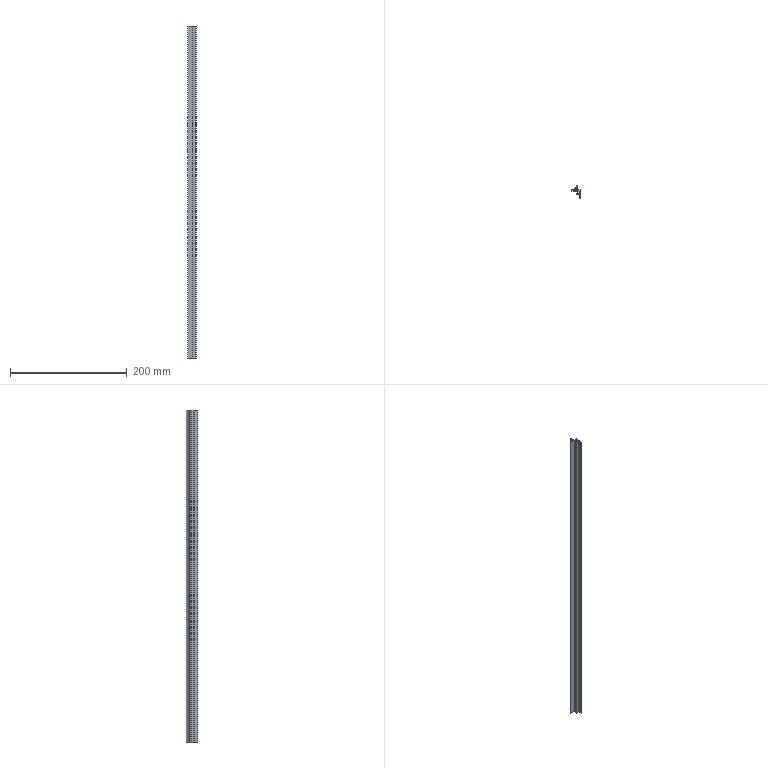Part | SolidWorks | features BaseBody 1, ICE 1, MoveFace 1 | 1 solid | 27 faces | box 14 x 20.3 x 568 mm | volume 28920 mm3 | plane 20 | cylinder 7 | commonest cylinder face diameters 0.387 x2 0.8 x2 0.4 x1 20 x1 22 x1
STEP:
#1=CARTESIAN_POINT('',(-5.304,-0.625,200.));
#2=VERTEX_POINT('',#1);
#3=CARTESIAN_POINT('',(-5.449,-0.8125,200.));
#4=VERTEX_POINT('',#3);
#5=CARTESIAN_POINT('',(-5.255,-0.8125,200.));
#6=DIRECTION('',(0.,0.,1.));
#7=DIRECTION('',(-1.,0.,0.));
#8=AXIS2_PLACEMENT_3D('',#5,#6,#7);
#9=CIRCLE('',#8,0.1937);
#10=EDGE_CURVE('',#2,#4,#9,.T.);
#11=ORIENTED_EDGE('',*,*,#10,.T.);
#12=CARTESIAN_POINT('',(-5.449,-0.8125,-368.));
#13=VERTEX_POINT('',#12);
#14=CARTESIAN_POINT('',(-5.449,-0.8125,230.));
#15=DIRECTION('',(0.,0.,-1.));
#16=VECTOR('',#15,1000.);
#17=LINE('',#14,#16);
#18=EDGE_CURVE('',#4,#13,#17,.T.);
#19=ORIENTED_EDGE('',*,*,#18,.T.);
#20=CARTESIAN_POINT('',(-5.304,-0.625,-368.));
#21=VERTEX_POINT('',#20);
#22=CARTESIAN_POINT('',(-5.255,-0.8125,-368.));
#23=DIRECTION('',(0.,0.,-1.));
#24=DIRECTION('',(1.,0.,0.));
#25=AXIS2_PLACEMENT_3D('',#22,#23,#24);
#26=CIRCLE('',#25,0.1937);
#27=EDGE_CURVE('',#13,#21,#26,.T.);
#28=ORIENTED_EDGE('',*,*,#27,.T.);
#29=CARTESIAN_POINT('',(-5.304,-0.625,230.));
#30=DIRECTION('',(0.,0.,-1.));
#31=VECTOR('',#30,1000.);
#32=LINE('',#29,#31);
#33=EDGE_CURVE('',#2,#21,#32,.T.);
#34=ORIENTED_EDGE('',*,*,#33,.F.);
#35=EDGE_LOOP('',(#11,#19,#28,#34));
#36=FACE_OUTER_BOUND('',#35,.T.);
#37=CARTESIAN_POINT('',(-5.255,-0.8125,230.));
#38=DIRECTION('',(0.,0.,-1.));
#39=DIRECTION('',(-1.,0.,0.));
#40=AXIS2_PLACEMENT_3D('',#37,#38,#39);
#41=CYLINDRICAL_SURFACE('',#40,0.1937);
#42=ADVANCED_FACE('',(#36),#41,.F.);
#43=CARTESIAN_POINT('',(5.,-1.,-368.));
#44=VERTEX_POINT('',#43);
#45=CARTESIAN_POINT('',(5.,-14.3,-368.));
#46=VERTEX_POINT('',#45);
#47=CARTESIAN_POINT('',(5.,29.623,-368.));
#48=DIRECTION('',(0.,-1.,0.));
#49=VECTOR('',#48,1000.);
#50=LINE('',#47,#49);
#51=EDGE_CURVE('',#44,#46,#50,.T.);
#52=ORIENTED_EDGE('',*,*,#51,.F.);
#53=CARTESIAN_POINT('',(5.,-1.,200.));
#54=VERTEX_POINT('',#53);
#55=CARTESIAN_POINT('',(5.,-1.,230.));
#56=DIRECTION('',(0.,0.,-1.));
#57=VECTOR('',#56,1000.);
#58=LINE('',#55,#57);
#59=EDGE_CURVE('',#54,#44,#58,.T.);
#60=ORIENTED_EDGE('',*,*,#59,.F.);
#61=CARTESIAN_POINT('',(5.,-14.3,200.));
#62=VERTEX_POINT('',#61);
#63=CARTESIAN_POINT('',(5.,-14.3,200.));
#64=DIRECTION('',(0.,1.,0.));
#65=VECTOR('',#64,1000.);
#66=LINE('',#63,#65);
#67=EDGE_CURVE('',#62,#54,#66,.T.);
#68=ORIENTED_EDGE('',*,*,#67,.F.);
#69=CARTESIAN_POINT('',(5.,-14.3,230.));
#70=DIRECTION('',(0.,0.,1.));
#71=VECTOR('',#70,1000.);
#72=LINE('',#69,#71);
#73=EDGE_CURVE('',#46,#62,#72,.T.);
#74=ORIENTED_EDGE('',*,*,#73,.F.);
#75=EDGE_LOOP('',(#52,#60,#68,#74));
#76=FACE_OUTER_BOUND('',#75,.T.);
#77=CARTESIAN_POINT('',(5.,-14.3,230.));
#78=DIRECTION('',(-1.,0.,0.));
#79=DIRECTION('',(0.,0.,1.));
#80=AXIS2_PLACEMENT_3D('',#77,#78,#79);
#81=PLANE('',#80);
#82=ADVANCED_FACE('',(#76),#81,.F.);
#83=CARTESIAN_POINT('',(-9.,-2.,-368.));
#84=VERTEX_POINT('',#83);
#85=CARTESIAN_POINT('',(-9.,-2.,200.));
#86=VERTEX_POINT('',#85);
#87=CARTESIAN_POINT('',(-9.,-2.,230.));
#88=DIRECTION('',(0.,0.,1.));
#89=VECTOR('',#88,1000.);
#90=LINE('',#87,#89);
#91=EDGE_CURVE('',#84,#86,#90,.T.);
#92=ORIENTED_EDGE('',*,*,#91,.F.);
#93=CARTESIAN_POINT('',(0.9,-2.,-368.));
#94=VERTEX_POINT('',#93);
#95=CARTESIAN_POINT('',(5.,-2.,-368.));
#96=DIRECTION('',(-1.,0.,0.));
#97=VECTOR('',#96,1000.);
#98=LINE('',#95,#97);
#99=EDGE_CURVE('',#94,#84,#98,.T.);
#100=ORIENTED_EDGE('',*,*,#99,.F.);
#101=CARTESIAN_POINT('',(0.9,-2.,200.));
#102=VERTEX_POINT('',#101);
#103=CARTESIAN_POINT('',(0.9,-2.,230.));
#104=DIRECTION('',(0.,0.,-1.));
#105=VECTOR('',#104,1000.);
#106=LINE('',#103,#105);
#107=EDGE_CURVE('',#102,#94,#106,.T.);
#108=ORIENTED_EDGE('',*,*,#107,.F.);
#109=CARTESIAN_POINT('',(5.,-2.,200.));
#110=DIRECTION('',(1.,0.,0.));
#111=VECTOR('',#110,1000.);
#112=LINE('',#109,#111);
#113=EDGE_CURVE('',#86,#102,#112,.T.);
#114=ORIENTED_EDGE('',*,*,#113,.F.);
#115=EDGE_LOOP('',(#92,#100,#108,#114));
#116=FACE_OUTER_BOUND('',#115,.T.);
#117=CARTESIAN_POINT('',(-9.,-2.,230.));
#118=DIRECTION('',(0.,1.,0.));
#119=DIRECTION('',(0.,0.,1.));
#120=AXIS2_PLACEMENT_3D('',#117,#118,#119);
#121=PLANE('',#120);
#122=ADVANCED_FACE('',(#116),#121,.F.);
#123=CARTESIAN_POINT('',(4.,-6.,200.));
#124=VERTEX_POINT('',#123);
#125=CARTESIAN_POINT('',(4.,-3.,200.));
#126=VERTEX_POINT('',#125);
#127=CARTESIAN_POINT('',(4.,29.623,200.));
#128=DIRECTION('',(0.,1.,0.));
#129=VECTOR('',#128,1000.);
#130=LINE('',#127,#129);
#131=EDGE_CURVE('',#124,#126,#130,.T.);
#132=ORIENTED_EDGE('',*,*,#131,.F.);
#133=CARTESIAN_POINT('',(1.,-6.,200.));
#134=VERTEX_POINT('',#133);
#135=CARTESIAN_POINT('',(5.,-6.,200.));
#136=DIRECTION('',(1.,0.,0.));
#137=VECTOR('',#136,1000.);
#138=LINE('',#135,#137);
#139=EDGE_CURVE('',#134,#124,#138,.T.);
#140=ORIENTED_EDGE('',*,*,#139,.F.);
#141=CARTESIAN_POINT('',(1.,-6.7,200.));
#142=VERTEX_POINT('',#141);
#143=CARTESIAN_POINT('',(1.,-6.,200.));
#144=DIRECTION('',(0.,-1.,0.));
#145=VECTOR('',#144,1000.);
#146=LINE('',#143,#145);
#147=EDGE_CURVE('',#134,#142,#146,.T.);
#148=ORIENTED_EDGE('',*,*,#147,.T.);
#149=CARTESIAN_POINT('',(-1.7,-6.7,200.));
#150=VERTEX_POINT('',#149);
#151=CARTESIAN_POINT('',(5.,-6.7,200.));
#152=DIRECTION('',(1.,0.,0.));
#153=VECTOR('',#152,1000.);
#154=LINE('',#151,#153);
#155=EDGE_CURVE('',#150,#142,#154,.T.);
#156=ORIENTED_EDGE('',*,*,#155,.F.);
#157=CARTESIAN_POINT('',(-1.7,-7.7,200.));
#158=VERTEX_POINT('',#157);
#159=CARTESIAN_POINT('',(-1.7,-6.7,200.));
#160=DIRECTION('',(0.,-1.,0.));
#161=VECTOR('',#160,1000.);
#162=LINE('',#159,#161);
#163=EDGE_CURVE('',#150,#158,#162,.T.);
#164=ORIENTED_EDGE('',*,*,#163,.T.);
#165=CARTESIAN_POINT('',(4.,-7.7,200.));
#166=VERTEX_POINT('',#165);
#167=CARTESIAN_POINT('',(5.,-7.7,200.));
#168=DIRECTION('',(-1.,0.,0.));
#169=VECTOR('',#168,1000.);
#170=LINE('',#167,#169);
#171=EDGE_CURVE('',#166,#158,#170,.T.);
#172=ORIENTED_EDGE('',*,*,#171,.F.);
#173=CARTESIAN_POINT('',(4.,-14.3,200.));
#174=VERTEX_POINT('',#173);
#175=CARTESIAN_POINT('',(4.,29.623,200.));
#176=DIRECTION('',(0.,1.,0.));
#177=VECTOR('',#176,1000.);
#178=LINE('',#175,#177);
#179=EDGE_CURVE('',#174,#166,#178,.T.);
#180=ORIENTED_EDGE('',*,*,#179,.F.);
#181=CARTESIAN_POINT('',(5.,-14.3,200.));
#182=DIRECTION('',(-1.,0.,0.));
#183=VECTOR('',#182,1000.);
#184=LINE('',#181,#183);
#185=EDGE_CURVE('',#62,#174,#184,.T.);
#186=ORIENTED_EDGE('',*,*,#185,.F.);
#187=ORIENTED_EDGE('',*,*,#67,.T.);
#188=CARTESIAN_POINT('',(-5.207,-1.,200.));
#189=VERTEX_POINT('',#188);
#190=CARTESIAN_POINT('',(5.,-1.,200.));
#191=DIRECTION('',(1.,0.,0.));
#192=VECTOR('',#191,1000.);
#193=LINE('',#190,#192);
#194=EDGE_CURVE('',#189,#54,#193,.T.);
#195=ORIENTED_EDGE('',*,*,#194,.F.);
#196=CARTESIAN_POINT('',(-5.255,-0.8125,200.));
#197=DIRECTION('',(0.,0.,1.));
#198=DIRECTION('',(-1.,0.,0.));
#199=AXIS2_PLACEMENT_3D('',#196,#197,#198);
#200=CIRCLE('',#199,0.1937);
#201=EDGE_CURVE('',#4,#189,#200,.T.);
#202=ORIENTED_EDGE('',*,*,#201,.F.);
#203=ORIENTED_EDGE('',*,*,#10,.F.);
#204=CARTESIAN_POINT('',(-1.368,3.063,200.));
#205=VERTEX_POINT('',#204);
#206=CARTESIAN_POINT('',(-10.628,9.,200.));
#207=DIRECTION('',(0.,0.,1.));
#208=DIRECTION('',(-1.,0.,0.));
#209=AXIS2_PLACEMENT_3D('',#206,#207,#208);
#210=CIRCLE('',#209,11.);
#211=EDGE_CURVE('',#2,#205,#210,.T.);
#212=ORIENTED_EDGE('',*,*,#211,.T.);
#213=CARTESIAN_POINT('',(-1.,2.955,200.));
#214=VERTEX_POINT('',#213);
#215=CARTESIAN_POINT('',(-1.2,2.955,200.));
#216=DIRECTION('',(0.,0.,1.));
#217=DIRECTION('',(-1.,0.,0.));
#218=AXIS2_PLACEMENT_3D('',#215,#216,#217);
#219=CIRCLE('',#218,0.2);
#220=EDGE_CURVE('',#214,#205,#219,.T.);
#221=ORIENTED_EDGE('',*,*,#220,.F.);
#222=CARTESIAN_POINT('',(-1.,1.5,200.));
#223=VERTEX_POINT('',#222);
#224=CARTESIAN_POINT('',(-1.,2.955,200.));
#225=DIRECTION('',(0.,1.,0.));
#226=VECTOR('',#225,1000.);
#227=LINE('',#224,#226);
#228=EDGE_CURVE('',#223,#214,#227,.T.);
#229=ORIENTED_EDGE('',*,*,#228,.F.);
#230=CARTESIAN_POINT('',(0.,1.5,200.));
#231=VERTEX_POINT('',#230);
#232=CARTESIAN_POINT('',(-1.,1.5,200.));
#233=DIRECTION('',(-1.,0.,0.));
#234=VECTOR('',#233,1000.);
#235=LINE('',#232,#234);
#236=EDGE_CURVE('',#231,#223,#235,.T.);
#237=ORIENTED_EDGE('',*,*,#236,.F.);
#238=CARTESIAN_POINT('',(0.,6.,200.));
#239=VERTEX_POINT('',#238);
#240=CARTESIAN_POINT('',(0.,1.5,200.));
#241=DIRECTION('',(0.,-1.,0.));
#242=VECTOR('',#241,1000.);
#243=LINE('',#240,#242);
#244=EDGE_CURVE('',#239,#231,#243,.T.);
#245=ORIENTED_EDGE('',*,*,#244,.F.);
#246=CARTESIAN_POINT('',(-0.8,6.,200.));
#247=VERTEX_POINT('',#246);
#248=CARTESIAN_POINT('',(0.,6.,200.));
#249=DIRECTION('',(1.,0.,0.));
#250=VECTOR('',#249,1000.);
#251=LINE('',#248,#250);
#252=EDGE_CURVE('',#247,#239,#251,.T.);
#253=ORIENTED_EDGE('',*,*,#252,.F.);
#254=CARTESIAN_POINT('',(-1.178,5.731,200.));
#255=VERTEX_POINT('',#254);
#256=CARTESIAN_POINT('',(-0.8,5.6,200.));
#257=DIRECTION('',(0.,0.,1.));
#258=DIRECTION('',(-1.,0.,0.));
#259=AXIS2_PLACEMENT_3D('',#256,#257,#258);
#260=CIRCLE('',#259,0.4);
#261=EDGE_CURVE('',#247,#255,#260,.T.);
#262=ORIENTED_EDGE('',*,*,#261,.T.);
#263=CARTESIAN_POINT('',(-8.678,-0.8077,200.));
#264=VERTEX_POINT('',#263);
#265=CARTESIAN_POINT('',(-10.628,9.,200.));
#266=DIRECTION('',(0.,0.,1.));
#267=DIRECTION('',(-1.,0.,0.));
#268=AXIS2_PLACEMENT_3D('',#265,#266,#267);
#269=CIRCLE('',#268,10.);
#270=EDGE_CURVE('',#264,#255,#269,.T.);
#271=ORIENTED_EDGE('',*,*,#270,.F.);
#272=CARTESIAN_POINT('',(-9.,-1.2,200.));
#273=VERTEX_POINT('',#272);
#274=CARTESIAN_POINT('',(-8.6,-1.2,200.));
#275=DIRECTION('',(0.,0.,1.));
#276=DIRECTION('',(-1.,0.,0.));
#277=AXIS2_PLACEMENT_3D('',#274,#275,#276);
#278=CIRCLE('',#277,0.4);
#279=EDGE_CURVE('',#264,#273,#278,.T.);
#280=ORIENTED_EDGE('',*,*,#279,.T.);
#281=CARTESIAN_POINT('',(-9.,8.,200.));
#282=DIRECTION('',(0.,-1.,0.));
#283=VECTOR('',#282,1000.);
#284=LINE('',#281,#283);
#285=EDGE_CURVE('',#273,#86,#284,.T.);
#286=ORIENTED_EDGE('',*,*,#285,.T.);
#287=ORIENTED_EDGE('',*,*,#113,.T.);
#288=CARTESIAN_POINT('',(0.9,-3.,200.));
#289=VERTEX_POINT('',#288);
#290=CARTESIAN_POINT('',(0.9,29.623,200.));
#291=DIRECTION('',(0.,1.,0.));
#292=VECTOR('',#291,1000.);
#293=LINE('',#290,#292);
#294=EDGE_CURVE('',#289,#102,#293,.T.);
#295=ORIENTED_EDGE('',*,*,#294,.F.);
#296=CARTESIAN_POINT('',(5.,-3.,200.));
#297=DIRECTION('',(-1.,0.,0.));
#298=VECTOR('',#297,1000.);
#299=LINE('',#296,#298);
#300=EDGE_CURVE('',#126,#289,#299,.T.);
#301=ORIENTED_EDGE('',*,*,#300,.F.);
#302=EDGE_LOOP('',(#132,#140,#148,#156,#164,#172,#180,#186,#187,#195,#202,#203,#212,#221,#229,#237,#245,#253,#262,#271,#280,#286,#287,#295,#301));
#303=FACE_OUTER_BOUND('',#302,.T.);
#304=CARTESIAN_POINT('',(5.,29.623,200.));
#305=DIRECTION('',(0.,0.,-1.));
#306=DIRECTION('',(-1.,0.,0.));
#307=AXIS2_PLACEMENT_3D('',#304,#305,#306);
#308=PLANE('',#307);
#309=ADVANCED_FACE('',(#303),#308,.F.);
#310=ORIENTED_EDGE('',*,*,#185,.T.);
#311=CARTESIAN_POINT('',(4.,-14.3,-368.));
#312=VERTEX_POINT('',#311);
#313=CARTESIAN_POINT('',(4.,-14.3,230.));
#314=DIRECTION('',(0.,0.,1.));
#315=VECTOR('',#314,1000.);
#316=LINE('',#313,#315);
#317=EDGE_CURVE('',#312,#174,#316,.T.);
#318=ORIENTED_EDGE('',*,*,#317,.F.);
#319=CARTESIAN_POINT('',(5.,-14.3,-368.));
#320=DIRECTION('',(-1.,0.,0.));
#321=VECTOR('',#320,1000.);
#322=LINE('',#319,#321);
#323=EDGE_CURVE('',#46,#312,#322,.T.);
#324=ORIENTED_EDGE('',*,*,#323,.F.);
#325=ORIENTED_EDGE('',*,*,#73,.T.);
#326=EDGE_LOOP('',(#310,#318,#324,#325));
#327=FACE_OUTER_BOUND('',#326,.T.);
#328=CARTESIAN_POINT('',(4.,-14.3,230.));
#329=DIRECTION('',(0.,1.,0.));
#330=DIRECTION('',(0.,0.,1.));
#331=AXIS2_PLACEMENT_3D('',#328,#329,#330);
#332=PLANE('',#331);
#333=ADVANCED_FACE('',(#327),#332,.F.);
#334=ORIENTED_EDGE('',*,*,#51,.T.);
#335=ORIENTED_EDGE('',*,*,#323,.T.);
#336=CARTESIAN_POINT('',(4.,-7.7,-368.));
#337=VERTEX_POINT('',#336);
#338=CARTESIAN_POINT('',(4.,-7.7,-368.));
#339=DIRECTION('',(0.,-1.,0.));
#340=VECTOR('',#339,1000.);
#341=LINE('',#338,#340);
#342=EDGE_CURVE('',#337,#312,#341,.T.);
#343=ORIENTED_EDGE('',*,*,#342,.F.);
#344=CARTESIAN_POINT('',(-1.7,-7.7,-368.));
#345=VERTEX_POINT('',#344);
#346=CARTESIAN_POINT('',(-1.7,-7.7,-368.));
#347=DIRECTION('',(1.,0.,0.));
#348=VECTOR('',#347,1000.);
#349=LINE('',#346,#348);
#350=EDGE_CURVE('',#345,#337,#349,.T.);
#351=ORIENTED_EDGE('',*,*,#350,.F.);
#352=CARTESIAN_POINT('',(-1.7,-6.7,-368.));
#353=VERTEX_POINT('',#352);
#354=CARTESIAN_POINT('',(-1.7,29.623,-368.));
#355=DIRECTION('',(0.,1.,0.));
#356=VECTOR('',#355,1000.);
#357=LINE('',#354,#356);
#358=EDGE_CURVE('',#345,#353,#357,.T.);
#359=ORIENTED_EDGE('',*,*,#358,.T.);
#360=CARTESIAN_POINT('',(1.,-6.7,-368.));
#361=VERTEX_POINT('',#360);
#362=CARTESIAN_POINT('',(1.,-6.7,-368.));
#363=DIRECTION('',(-1.,0.,0.));
#364=VECTOR('',#363,1000.);
#365=LINE('',#362,#364);
#366=EDGE_CURVE('',#361,#353,#365,.T.);
#367=ORIENTED_EDGE('',*,*,#366,.F.);
#368=CARTESIAN_POINT('',(1.,-6.,-368.));
#369=VERTEX_POINT('',#368);
#370=CARTESIAN_POINT('',(1.,29.623,-368.));
#371=DIRECTION('',(0.,1.,0.));
#372=VECTOR('',#371,1000.);
#373=LINE('',#370,#372);
#374=EDGE_CURVE('',#361,#369,#373,.T.);
#375=ORIENTED_EDGE('',*,*,#374,.T.);
#376=CARTESIAN_POINT('',(4.,-6.,-368.));
#377=VERTEX_POINT('',#376);
#378=CARTESIAN_POINT('',(4.,-6.,-368.));
#379=DIRECTION('',(-1.,0.,0.));
#380=VECTOR('',#379,1000.);
#381=LINE('',#378,#380);
#382=EDGE_CURVE('',#377,#369,#381,.T.);
#383=ORIENTED_EDGE('',*,*,#382,.F.);
#384=CARTESIAN_POINT('',(4.,-3.,-368.));
#385=VERTEX_POINT('',#384);
#386=CARTESIAN_POINT('',(4.,-3.,-368.));
#387=DIRECTION('',(0.,-1.,0.));
#388=VECTOR('',#387,1000.);
#389=LINE('',#386,#388);
#390=EDGE_CURVE('',#385,#377,#389,.T.);
#391=ORIENTED_EDGE('',*,*,#390,.F.);
#392=CARTESIAN_POINT('',(0.9,-3.,-368.));
#393=VERTEX_POINT('',#392);
#394=CARTESIAN_POINT('',(0.9,-3.,-368.));
#395=DIRECTION('',(1.,0.,0.));
#396=VECTOR('',#395,1000.);
#397=LINE('',#394,#396);
#398=EDGE_CURVE('',#393,#385,#397,.T.);
#399=ORIENTED_EDGE('',*,*,#398,.F.);
#400=CARTESIAN_POINT('',(0.9,-2.,-368.));
#401=DIRECTION('',(0.,-1.,0.));
#402=VECTOR('',#401,1000.);
#403=LINE('',#400,#402);
#404=EDGE_CURVE('',#94,#393,#403,.T.);
#405=ORIENTED_EDGE('',*,*,#404,.F.);
#406=ORIENTED_EDGE('',*,*,#99,.T.);
#407=CARTESIAN_POINT('',(-9.,-1.2,-368.));
#408=VERTEX_POINT('',#407);
#409=CARTESIAN_POINT('',(-9.,-1.2,-368.));
#410=DIRECTION('',(0.,-1.,0.));
#411=VECTOR('',#410,1000.);
#412=LINE('',#409,#411);
#413=EDGE_CURVE('',#408,#84,#412,.T.);
#414=ORIENTED_EDGE('',*,*,#413,.F.);
#415=CARTESIAN_POINT('',(-8.678,-0.8077,-368.));
#416=VERTEX_POINT('',#415);
#417=CARTESIAN_POINT('',(-8.6,-1.2,-368.));
#418=DIRECTION('',(0.,0.,-1.));
#419=DIRECTION('',(1.,0.,0.));
#420=AXIS2_PLACEMENT_3D('',#417,#418,#419);
#421=CIRCLE('',#420,0.4);
#422=EDGE_CURVE('',#408,#416,#421,.T.);
#423=ORIENTED_EDGE('',*,*,#422,.T.);
#424=CARTESIAN_POINT('',(-1.178,5.731,-368.));
#425=VERTEX_POINT('',#424);
#426=CARTESIAN_POINT('',(-10.628,9.,-368.));
#427=DIRECTION('',(0.,0.,-1.));
#428=DIRECTION('',(1.,0.,0.));
#429=AXIS2_PLACEMENT_3D('',#426,#427,#428);
#430=CIRCLE('',#429,10.);
#431=EDGE_CURVE('',#425,#416,#430,.T.);
#432=ORIENTED_EDGE('',*,*,#431,.F.);
#433=CARTESIAN_POINT('',(-0.8,6.,-368.));
#434=VERTEX_POINT('',#433);
#435=CARTESIAN_POINT('',(-0.8,5.6,-368.));
#436=DIRECTION('',(0.,0.,-1.));
#437=DIRECTION('',(1.,0.,0.));
#438=AXIS2_PLACEMENT_3D('',#435,#436,#437);
#439=CIRCLE('',#438,0.4);
#440=EDGE_CURVE('',#425,#434,#439,.T.);
#441=ORIENTED_EDGE('',*,*,#440,.T.);
#442=CARTESIAN_POINT('',(0.,6.,-368.));
#443=VERTEX_POINT('',#442);
#444=CARTESIAN_POINT('',(0.,6.,-368.));
#445=DIRECTION('',(-1.,0.,0.));
#446=VECTOR('',#445,1000.);
#447=LINE('',#444,#446);
#448=EDGE_CURVE('',#443,#434,#447,.T.);
#449=ORIENTED_EDGE('',*,*,#448,.F.);
#450=CARTESIAN_POINT('',(0.,1.5,-368.));
#451=VERTEX_POINT('',#450);
#452=CARTESIAN_POINT('',(0.,1.5,-368.));
#453=DIRECTION('',(0.,1.,0.));
#454=VECTOR('',#453,1000.);
#455=LINE('',#452,#454);
#456=EDGE_CURVE('',#451,#443,#455,.T.);
#457=ORIENTED_EDGE('',*,*,#456,.F.);
#458=CARTESIAN_POINT('',(-1.,1.5,-368.));
#459=VERTEX_POINT('',#458);
#460=CARTESIAN_POINT('',(-1.,1.5,-368.));
#461=DIRECTION('',(1.,0.,0.));
#462=VECTOR('',#461,1000.);
#463=LINE('',#460,#462);
#464=EDGE_CURVE('',#459,#451,#463,.T.);
#465=ORIENTED_EDGE('',*,*,#464,.F.);
#466=CARTESIAN_POINT('',(-1.,2.955,-368.));
#467=VERTEX_POINT('',#466);
#468=CARTESIAN_POINT('',(-1.,2.955,-368.));
#469=DIRECTION('',(0.,-1.,0.));
#470=VECTOR('',#469,1000.);
#471=LINE('',#468,#470);
#472=EDGE_CURVE('',#467,#459,#471,.T.);
#473=ORIENTED_EDGE('',*,*,#472,.F.);
#474=CARTESIAN_POINT('',(-1.368,3.063,-368.));
#475=VERTEX_POINT('',#474);
#476=CARTESIAN_POINT('',(-1.2,2.955,-368.));
#477=DIRECTION('',(0.,0.,-1.));
#478=DIRECTION('',(1.,0.,0.));
#479=AXIS2_PLACEMENT_3D('',#476,#477,#478);
#480=CIRCLE('',#479,0.2);
#481=EDGE_CURVE('',#475,#467,#480,.T.);
#482=ORIENTED_EDGE('',*,*,#481,.F.);
#483=CARTESIAN_POINT('',(-10.628,9.,-368.));
#484=DIRECTION('',(0.,0.,-1.));
#485=DIRECTION('',(1.,0.,0.));
#486=AXIS2_PLACEMENT_3D('',#483,#484,#485);
#487=CIRCLE('',#486,11.);
#488=EDGE_CURVE('',#475,#21,#487,.T.);
#489=ORIENTED_EDGE('',*,*,#488,.T.);
#490=ORIENTED_EDGE('',*,*,#27,.F.);
#491=CARTESIAN_POINT('',(-5.207,-1.,-368.));
#492=VERTEX_POINT('',#491);
#493=CARTESIAN_POINT('',(-5.255,-0.8125,-368.));
#494=DIRECTION('',(0.,0.,-1.));
#495=DIRECTION('',(1.,0.,0.));
#496=AXIS2_PLACEMENT_3D('',#493,#494,#495);
#497=CIRCLE('',#496,0.1937);
#498=EDGE_CURVE('',#492,#13,#497,.T.);
#499=ORIENTED_EDGE('',*,*,#498,.F.);
#500=CARTESIAN_POINT('',(5.,-1.,-368.));
#501=DIRECTION('',(-1.,0.,0.));
#502=VECTOR('',#501,1000.);
#503=LINE('',#500,#502);
#504=EDGE_CURVE('',#44,#492,#503,.T.);
#505=ORIENTED_EDGE('',*,*,#504,.F.);
#506=EDGE_LOOP('',(#334,#335,#343,#351,#359,#367,#375,#383,#391,#399,#405,#406,#414,#423,#432,#441,#449,#457,#465,#473,#482,#489,#490,#499,#505));
#507=FACE_OUTER_BOUND('',#506,.T.);
#508=CARTESIAN_POINT('',(5.,29.623,-368.));
#509=DIRECTION('',(0.,0.,1.));
#510=DIRECTION('',(1.,0.,0.));
#511=AXIS2_PLACEMENT_3D('',#508,#509,#510);
#512=PLANE('',#511);
#513=ADVANCED_FACE('',(#507),#512,.F.);
#514=ORIENTED_EDGE('',*,*,#59,.T.);
#515=ORIENTED_EDGE('',*,*,#504,.T.);
#516=CARTESIAN_POINT('',(-5.207,-1.,230.));
#517=DIRECTION('',(0.,0.,-1.));
#518=VECTOR('',#517,1000.);
#519=LINE('',#516,#518);
#520=EDGE_CURVE('',#189,#492,#519,.T.);
#521=ORIENTED_EDGE('',*,*,#520,.F.);
#522=ORIENTED_EDGE('',*,*,#194,.T.);
#523=EDGE_LOOP('',(#514,#515,#521,#522));
#524=FACE_OUTER_BOUND('',#523,.T.);
#525=CARTESIAN_POINT('',(5.,-1.,230.));
#526=DIRECTION('',(0.,-1.,0.));
#527=DIRECTION('',(0.,0.,-1.));
#528=AXIS2_PLACEMENT_3D('',#525,#526,#527);
#529=PLANE('',#528);
#530=ADVANCED_FACE('',(#524),#529,.F.);
#531=CARTESIAN_POINT('',(-9.,-1.2,230.));
#532=DIRECTION('',(0.,0.,1.));
#533=VECTOR('',#532,1000.);
#534=LINE('',#531,#533);
#535=EDGE_CURVE('',#408,#273,#534,.T.);
#536=ORIENTED_EDGE('',*,*,#535,.F.);
#537=ORIENTED_EDGE('',*,*,#413,.T.);
#538=ORIENTED_EDGE('',*,*,#91,.T.);
#539=ORIENTED_EDGE('',*,*,#285,.F.);
#540=EDGE_LOOP('',(#536,#537,#538,#539));
#541=FACE_OUTER_BOUND('',#540,.T.);
#542=CARTESIAN_POINT('',(-9.,-1.2,230.));
#543=DIRECTION('',(1.,0.,0.));
#544=DIRECTION('',(0.,0.,-1.));
#545=AXIS2_PLACEMENT_3D('',#542,#543,#544);
#546=PLANE('',#545);
#547=ADVANCED_FACE('',(#541),#546,.F.);
#548=ORIENTED_EDGE('',*,*,#294,.T.);
#549=ORIENTED_EDGE('',*,*,#107,.T.);
#550=ORIENTED_EDGE('',*,*,#404,.T.);
#551=CARTESIAN_POINT('',(0.9,-3.,230.));
#552=DIRECTION('',(0.,0.,-1.));
#553=VECTOR('',#552,1000.);
#554=LINE('',#551,#553);
#555=EDGE_CURVE('',#289,#393,#554,.T.);
#556=ORIENTED_EDGE('',*,*,#555,.F.);
#557=EDGE_LOOP('',(#548,#549,#550,#556));
#558=FACE_OUTER_BOUND('',#557,.T.);
#559=CARTESIAN_POINT('',(0.9,-2.,230.));
#560=DIRECTION('',(1.,0.,0.));
#561=DIRECTION('',(0.,0.,-1.));
#562=AXIS2_PLACEMENT_3D('',#559,#560,#561);
#563=PLANE('',#562);
#564=ADVANCED_FACE('',(#558),#563,.F.);
#565=ORIENTED_EDGE('',*,*,#300,.T.);
#566=ORIENTED_EDGE('',*,*,#555,.T.);
#567=ORIENTED_EDGE('',*,*,#398,.T.);
#568=CARTESIAN_POINT('',(4.,-3.,230.));
#569=DIRECTION('',(0.,0.,-1.));
#570=VECTOR('',#569,1000.);
#571=LINE('',#568,#570);
#572=EDGE_CURVE('',#126,#385,#571,.T.);
#573=ORIENTED_EDGE('',*,*,#572,.F.);
#574=EDGE_LOOP('',(#565,#566,#567,#573));
#575=FACE_OUTER_BOUND('',#574,.T.);
#576=CARTESIAN_POINT('',(0.9,-3.,230.));
#577=DIRECTION('',(0.,1.,0.));
#578=DIRECTION('',(0.,0.,1.));
#579=AXIS2_PLACEMENT_3D('',#576,#577,#578);
#580=PLANE('',#579);
#581=ADVANCED_FACE('',(#575),#580,.F.);
#582=ORIENTED_EDGE('',*,*,#131,.T.);
#583=ORIENTED_EDGE('',*,*,#572,.T.);
#584=ORIENTED_EDGE('',*,*,#390,.T.);
#585=CARTESIAN_POINT('',(4.,-6.,230.));
#586=DIRECTION('',(0.,0.,-1.));
#587=VECTOR('',#586,1000.);
#588=LINE('',#585,#587);
#589=EDGE_CURVE('',#124,#377,#588,.T.);
#590=ORIENTED_EDGE('',*,*,#589,.F.);
#591=EDGE_LOOP('',(#582,#583,#584,#590));
#592=FACE_OUTER_BOUND('',#591,.T.);
#593=CARTESIAN_POINT('',(4.,-3.,230.));
#594=DIRECTION('',(1.,0.,0.));
#595=DIRECTION('',(0.,0.,-1.));
#596=AXIS2_PLACEMENT_3D('',#593,#594,#595);
#597=PLANE('',#596);
#598=ADVANCED_FACE('',(#592),#597,.F.);
#599=ORIENTED_EDGE('',*,*,#139,.T.);
#600=ORIENTED_EDGE('',*,*,#589,.T.);
#601=ORIENTED_EDGE('',*,*,#382,.T.);
#602=CARTESIAN_POINT('',(1.,-6.,230.));
#603=DIRECTION('',(0.,0.,-1.));
#604=VECTOR('',#603,1000.);
#605=LINE('',#602,#604);
#606=EDGE_CURVE('',#134,#369,#605,.T.);
#607=ORIENTED_EDGE('',*,*,#606,.F.);
#608=EDGE_LOOP('',(#599,#600,#601,#607));
#609=FACE_OUTER_BOUND('',#608,.T.);
#610=CARTESIAN_POINT('',(4.,-6.,230.));
#611=DIRECTION('',(0.,-1.,0.));
#612=DIRECTION('',(0.,0.,-1.));
#613=AXIS2_PLACEMENT_3D('',#610,#611,#612);
#614=PLANE('',#613);
#615=ADVANCED_FACE('',(#609),#614,.F.);
#616=ORIENTED_EDGE('',*,*,#155,.T.);
#617=CARTESIAN_POINT('',(1.,-6.7,230.));
#618=DIRECTION('',(0.,0.,1.));
#619=VECTOR('',#618,1000.);
#620=LINE('',#617,#619);
#621=EDGE_CURVE('',#361,#142,#620,.T.);
#622=ORIENTED_EDGE('',*,*,#621,.F.);
#623=ORIENTED_EDGE('',*,*,#366,.T.);
#624=CARTESIAN_POINT('',(-1.7,-6.7,230.));
#625=DIRECTION('',(0.,0.,-1.));
#626=VECTOR('',#625,1000.);
#627=LINE('',#624,#626);
#628=EDGE_CURVE('',#150,#353,#627,.T.);
#629=ORIENTED_EDGE('',*,*,#628,.F.);
#630=EDGE_LOOP('',(#616,#622,#623,#629));
#631=FACE_OUTER_BOUND('',#630,.T.);
#632=CARTESIAN_POINT('',(1.,-6.7,230.));
#633=DIRECTION('',(0.,-1.,0.));
#634=DIRECTION('',(0.,0.,-1.));
#635=AXIS2_PLACEMENT_3D('',#632,#633,#634);
#636=PLANE('',#635);
#637=ADVANCED_FACE('',(#631),#636,.F.);
#638=ORIENTED_EDGE('',*,*,#171,.T.);
#639=CARTESIAN_POINT('',(-1.7,-7.7,230.));
#640=DIRECTION('',(0.,0.,1.));
#641=VECTOR('',#640,1000.);
#642=LINE('',#639,#641);
#643=EDGE_CURVE('',#345,#158,#642,.T.);
#644=ORIENTED_EDGE('',*,*,#643,.F.);
#645=ORIENTED_EDGE('',*,*,#350,.T.);
#646=CARTESIAN_POINT('',(4.,-7.7,230.));
#647=DIRECTION('',(0.,0.,-1.));
#648=VECTOR('',#647,1000.);
#649=LINE('',#646,#648);
#650=EDGE_CURVE('',#166,#337,#649,.T.);
#651=ORIENTED_EDGE('',*,*,#650,.F.);
#652=EDGE_LOOP('',(#638,#644,#645,#651));
#653=FACE_OUTER_BOUND('',#652,.T.);
#654=CARTESIAN_POINT('',(-1.7,-7.7,230.));
#655=DIRECTION('',(0.,1.,0.));
#656=DIRECTION('',(0.,0.,1.));
#657=AXIS2_PLACEMENT_3D('',#654,#655,#656);
#658=PLANE('',#657);
#659=ADVANCED_FACE('',(#653),#658,.F.);
#660=ORIENTED_EDGE('',*,*,#179,.T.);
#661=ORIENTED_EDGE('',*,*,#650,.T.);
#662=ORIENTED_EDGE('',*,*,#342,.T.);
#663=ORIENTED_EDGE('',*,*,#317,.T.);
#664=EDGE_LOOP('',(#660,#661,#662,#663));
#665=FACE_OUTER_BOUND('',#664,.T.);
#666=CARTESIAN_POINT('',(4.,-7.7,230.));
#667=DIRECTION('',(1.,0.,0.));
#668=DIRECTION('',(0.,0.,-1.));
#669=AXIS2_PLACEMENT_3D('',#666,#667,#668);
#670=PLANE('',#669);
#671=ADVANCED_FACE('',(#665),#670,.F.);
#672=ORIENTED_EDGE('',*,*,#18,.F.);
#673=ORIENTED_EDGE('',*,*,#201,.T.);
#674=ORIENTED_EDGE('',*,*,#520,.T.);
#675=ORIENTED_EDGE('',*,*,#498,.T.);
#676=EDGE_LOOP('',(#672,#673,#674,#675));
#677=FACE_OUTER_BOUND('',#676,.T.);
#678=CARTESIAN_POINT('',(-5.255,-0.8125,230.));
#679=DIRECTION('',(0.,0.,-1.));
#680=DIRECTION('',(-1.,0.,0.));
#681=AXIS2_PLACEMENT_3D('',#678,#679,#680);
#682=CYLINDRICAL_SURFACE('',#681,0.1937);
#683=ADVANCED_FACE('',(#677),#682,.F.);
#684=CARTESIAN_POINT('',(-1.,2.955,230.));
#685=DIRECTION('',(0.,0.,1.));
#686=VECTOR('',#685,1000.);
#687=LINE('',#684,#686);
#688=EDGE_CURVE('',#467,#214,#687,.T.);
#689=ORIENTED_EDGE('',*,*,#688,.F.);
#690=ORIENTED_EDGE('',*,*,#472,.T.);
#691=CARTESIAN_POINT('',(-1.,1.5,230.));
#692=DIRECTION('',(0.,0.,-1.));
#693=VECTOR('',#692,1000.);
#694=LINE('',#691,#693);
#695=EDGE_CURVE('',#223,#459,#694,.T.);
#696=ORIENTED_EDGE('',*,*,#695,.F.);
#697=ORIENTED_EDGE('',*,*,#228,.T.);
#698=EDGE_LOOP('',(#689,#690,#696,#697));
#699=FACE_OUTER_BOUND('',#698,.T.);
#700=CARTESIAN_POINT('',(-1.,2.955,230.));
#701=DIRECTION('',(1.,0.,0.));
#702=DIRECTION('',(0.,0.,-1.));
#703=AXIS2_PLACEMENT_3D('',#700,#701,#702);
#704=PLANE('',#703);
#705=ADVANCED_FACE('',(#699),#704,.F.);
#706=ORIENTED_EDGE('',*,*,#488,.F.);
#707=CARTESIAN_POINT('',(-1.368,3.063,230.));
#708=DIRECTION('',(0.,0.,1.));
#709=VECTOR('',#708,1000.);
#710=LINE('',#707,#709);
#711=EDGE_CURVE('',#475,#205,#710,.T.);
#712=ORIENTED_EDGE('',*,*,#711,.T.);
#713=ORIENTED_EDGE('',*,*,#211,.F.);
#714=ORIENTED_EDGE('',*,*,#33,.T.);
#715=EDGE_LOOP('',(#706,#712,#713,#714));
#716=FACE_OUTER_BOUND('',#715,.T.);
#717=CARTESIAN_POINT('',(-10.628,9.,230.));
#718=DIRECTION('',(0.,0.,-1.));
#719=DIRECTION('',(-1.,0.,0.));
#720=AXIS2_PLACEMENT_3D('',#717,#718,#719);
#721=CYLINDRICAL_SURFACE('',#720,11.);
#722=ADVANCED_FACE('',(#716),#721,.T.);
#723=CARTESIAN_POINT('',(-1.178,5.731,230.));
#724=DIRECTION('',(0.,0.,1.));
#725=VECTOR('',#724,1000.);
#726=LINE('',#723,#725);
#727=EDGE_CURVE('',#425,#255,#726,.T.);
#728=ORIENTED_EDGE('',*,*,#727,.F.);
#729=ORIENTED_EDGE('',*,*,#431,.T.);
#730=CARTESIAN_POINT('',(-8.678,-0.8077,230.));
#731=DIRECTION('',(0.,0.,-1.));
#732=VECTOR('',#731,1000.);
#733=LINE('',#730,#732);
#734=EDGE_CURVE('',#264,#416,#733,.T.);
#735=ORIENTED_EDGE('',*,*,#734,.F.);
#736=ORIENTED_EDGE('',*,*,#270,.T.);
#737=EDGE_LOOP('',(#728,#729,#735,#736));
#738=FACE_OUTER_BOUND('',#737,.T.);
#739=CARTESIAN_POINT('',(-10.628,9.,230.));
#740=DIRECTION('',(0.,0.,-1.));
#741=DIRECTION('',(-1.,0.,0.));
#742=AXIS2_PLACEMENT_3D('',#739,#740,#741);
#743=CYLINDRICAL_SURFACE('',#742,10.);
#744=ADVANCED_FACE('',(#738),#743,.F.);
#745=CARTESIAN_POINT('',(0.,1.5,230.));
#746=DIRECTION('',(0.,0.,1.));
#747=VECTOR('',#746,1000.);
#748=LINE('',#745,#747);
#749=EDGE_CURVE('',#451,#231,#748,.T.);
#750=ORIENTED_EDGE('',*,*,#749,.F.);
#751=ORIENTED_EDGE('',*,*,#456,.T.);
#752=CARTESIAN_POINT('',(0.,6.,230.));
#753=DIRECTION('',(0.,0.,-1.));
#754=VECTOR('',#753,1000.);
#755=LINE('',#752,#754);
#756=EDGE_CURVE('',#239,#443,#755,.T.);
#757=ORIENTED_EDGE('',*,*,#756,.F.);
#758=ORIENTED_EDGE('',*,*,#244,.T.);
#759=EDGE_LOOP('',(#750,#751,#757,#758));
#760=FACE_OUTER_BOUND('',#759,.T.);
#761=CARTESIAN_POINT('',(0.,1.5,230.));
#762=DIRECTION('',(-1.,0.,0.));
#763=DIRECTION('',(0.,0.,1.));
#764=AXIS2_PLACEMENT_3D('',#761,#762,#763);
#765=PLANE('',#764);
#766=ADVANCED_FACE('',(#760),#765,.F.);
#767=ORIENTED_EDGE('',*,*,#422,.F.);
#768=ORIENTED_EDGE('',*,*,#535,.T.);
#769=ORIENTED_EDGE('',*,*,#279,.F.);
#770=ORIENTED_EDGE('',*,*,#734,.T.);
#771=EDGE_LOOP('',(#767,#768,#769,#770));
#772=FACE_OUTER_BOUND('',#771,.T.);
#773=CARTESIAN_POINT('',(-8.6,-1.2,230.));
#774=DIRECTION('',(0.,0.,-1.));
#775=DIRECTION('',(-1.,0.,0.));
#776=AXIS2_PLACEMENT_3D('',#773,#774,#775);
#777=CYLINDRICAL_SURFACE('',#776,0.4);
#778=ADVANCED_FACE('',(#772),#777,.T.);
#779=ORIENTED_EDGE('',*,*,#147,.F.);
#780=ORIENTED_EDGE('',*,*,#606,.T.);
#781=ORIENTED_EDGE('',*,*,#374,.F.);
#782=ORIENTED_EDGE('',*,*,#621,.T.);
#783=EDGE_LOOP('',(#779,#780,#781,#782));
#784=FACE_OUTER_BOUND('',#783,.T.);
#785=CARTESIAN_POINT('',(1.,-6.,230.));
#786=DIRECTION('',(1.,0.,0.));
#787=DIRECTION('',(0.,0.,-1.));
#788=AXIS2_PLACEMENT_3D('',#785,#786,#787);
#789=PLANE('',#788);
#790=ADVANCED_FACE('',(#784),#789,.F.);
#791=ORIENTED_EDGE('',*,*,#163,.F.);
#792=ORIENTED_EDGE('',*,*,#628,.T.);
#793=ORIENTED_EDGE('',*,*,#358,.F.);
#794=ORIENTED_EDGE('',*,*,#643,.T.);
#795=EDGE_LOOP('',(#791,#792,#793,#794));
#796=FACE_OUTER_BOUND('',#795,.T.);
#797=CARTESIAN_POINT('',(-1.7,-6.7,230.));
#798=DIRECTION('',(1.,0.,0.));
#799=DIRECTION('',(0.,0.,-1.));
#800=AXIS2_PLACEMENT_3D('',#797,#798,#799);
#801=PLANE('',#800);
#802=ADVANCED_FACE('',(#796),#801,.F.);
#803=ORIENTED_EDGE('',*,*,#711,.F.);
#804=ORIENTED_EDGE('',*,*,#481,.T.);
#805=ORIENTED_EDGE('',*,*,#688,.T.);
#806=ORIENTED_EDGE('',*,*,#220,.T.);
#807=EDGE_LOOP('',(#803,#804,#805,#806));
#808=FACE_OUTER_BOUND('',#807,.T.);
#809=CARTESIAN_POINT('',(-1.2,2.955,230.));
#810=DIRECTION('',(0.,0.,-1.));
#811=DIRECTION('',(-1.,0.,0.));
#812=AXIS2_PLACEMENT_3D('',#809,#810,#811);
#813=CYLINDRICAL_SURFACE('',#812,0.2);
#814=ADVANCED_FACE('',(#808),#813,.F.);
#815=ORIENTED_EDGE('',*,*,#695,.T.);
#816=ORIENTED_EDGE('',*,*,#464,.T.);
#817=ORIENTED_EDGE('',*,*,#749,.T.);
#818=ORIENTED_EDGE('',*,*,#236,.T.);
#819=EDGE_LOOP('',(#815,#816,#817,#818));
#820=FACE_OUTER_BOUND('',#819,.T.);
#821=CARTESIAN_POINT('',(-1.,1.5,230.));
#822=DIRECTION('',(0.,1.,0.));
#823=DIRECTION('',(0.,0.,1.));
#824=AXIS2_PLACEMENT_3D('',#821,#822,#823);
#825=PLANE('',#824);
#826=ADVANCED_FACE('',(#820),#825,.F.);
#827=ORIENTED_EDGE('',*,*,#440,.F.);
#828=ORIENTED_EDGE('',*,*,#727,.T.);
#829=ORIENTED_EDGE('',*,*,#261,.F.);
#830=CARTESIAN_POINT('',(-0.8,6.,230.));
#831=DIRECTION('',(0.,0.,-1.));
#832=VECTOR('',#831,1000.);
#833=LINE('',#830,#832);
#834=EDGE_CURVE('',#247,#434,#833,.T.);
#835=ORIENTED_EDGE('',*,*,#834,.T.);
#836=EDGE_LOOP('',(#827,#828,#829,#835));
#837=FACE_OUTER_BOUND('',#836,.T.);
#838=CARTESIAN_POINT('',(-0.8,5.6,230.));
#839=DIRECTION('',(0.,0.,-1.));
#840=DIRECTION('',(-1.,0.,0.));
#841=AXIS2_PLACEMENT_3D('',#838,#839,#840);
#842=CYLINDRICAL_SURFACE('',#841,0.4);
#843=ADVANCED_FACE('',(#837),#842,.T.);
#844=ORIENTED_EDGE('',*,*,#756,.T.);
#845=ORIENTED_EDGE('',*,*,#448,.T.);
#846=ORIENTED_EDGE('',*,*,#834,.F.);
#847=ORIENTED_EDGE('',*,*,#252,.T.);
#848=EDGE_LOOP('',(#844,#845,#846,#847));
#849=FACE_OUTER_BOUND('',#848,.T.);
#850=CARTESIAN_POINT('',(0.,6.,230.));
#851=DIRECTION('',(0.,-1.,0.));
#852=DIRECTION('',(0.,0.,-1.));
#853=AXIS2_PLACEMENT_3D('',#850,#851,#852);
#854=PLANE('',#853);
#855=ADVANCED_FACE('',(#849),#854,.F.);
#856=CLOSED_SHELL('',(#42,#82,#122,#309,#333,#513,#530,#547,#564,#581,#598,#615,#637,#659,#671,#683,#705,#722,#744,#766,#778,#790,#802,#814,#826,#843,#855));
#857=MANIFOLD_SOLID_BREP('',#856);
#858=CARTESIAN_POINT('',(0.,0.,0.));
#859=DIRECTION('',(0.,0.,1.));
#860=DIRECTION('',(1.,0.,0.));
#861=AXIS2_PLACEMENT_3D('',#858,#859,#860);
#862=(LENGTH_UNIT()NAMED_UNIT(*)SI_UNIT(.MILLI.,.METRE.));
#863=UNCERTAINTY_MEASURE_WITH_UNIT(LENGTH_MEASURE(0.00001),#862,'','');
#864=(NAMED_UNIT(*)PLANE_ANGLE_UNIT()SI_UNIT($,.RADIAN.));
#865=(NAMED_UNIT(*)SI_UNIT($,.STERADIAN.)SOLID_ANGLE_UNIT());
#866=(GEOMETRIC_REPRESENTATION_CONTEXT(3)GLOBAL_UNCERTAINTY_ASSIGNED_CONTEXT((#863))GLOBAL_UNIT_ASSIGNED_CONTEXT((#862,#864,#865))REPRESENTATION_CONTEXT('',''));
#867=ADVANCED_BREP_SHAPE_REPRESENTATION('',(#857,#861),#866);